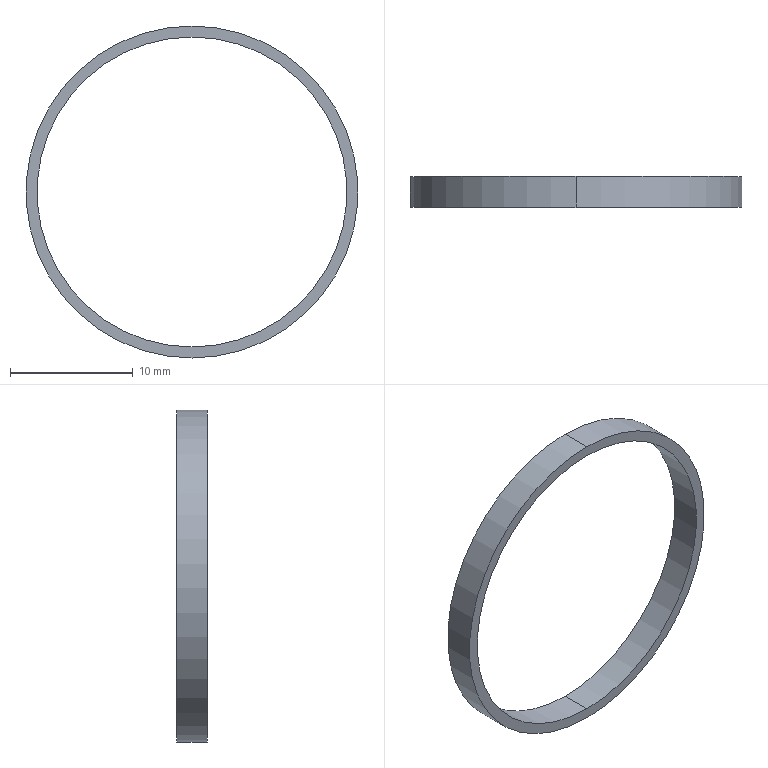Part | SolidWorks | features Extrusion 1 | 1 solid | 6 faces | box 27 x 2.5 x 27 mm | volume 184.49 mm3 | cylinder 4 | plane 2 | commonest cylinder face diameters 25.2 x2 27 x2
STEP:
#1=CARTESIAN_POINT('',(0.,2.5,-12.6));
#2=VERTEX_POINT('',#1);
#3=CARTESIAN_POINT('',(0.,2.5,12.6));
#4=VERTEX_POINT('',#3);
#5=CARTESIAN_POINT('',(0.,2.5,0.));
#6=DIRECTION('',(0.,1.,0.));
#7=DIRECTION('',(0.,0.,1.));
#8=AXIS2_PLACEMENT_3D('',#5,#6,#7);
#9=CIRCLE('',#8,12.6);
#10=EDGE_CURVE('',#2,#4,#9,.T.);
#11=ORIENTED_EDGE('',*,*,#10,.T.);
#12=CARTESIAN_POINT('',(0.,0.,12.6));
#13=VERTEX_POINT('',#12);
#14=CARTESIAN_POINT('',(0.,2.5,12.6));
#15=DIRECTION('',(0.,-1.,0.));
#16=VECTOR('',#15,1000.);
#17=LINE('',#14,#16);
#18=EDGE_CURVE('',#4,#13,#17,.T.);
#19=ORIENTED_EDGE('',*,*,#18,.T.);
#20=CARTESIAN_POINT('',(0.,0.,-12.6));
#21=VERTEX_POINT('',#20);
#22=CARTESIAN_POINT('',(0.,0.,0.));
#23=DIRECTION('',(0.,1.,0.));
#24=DIRECTION('',(0.,0.,1.));
#25=AXIS2_PLACEMENT_3D('',#22,#23,#24);
#26=CIRCLE('',#25,12.6);
#27=EDGE_CURVE('',#21,#13,#26,.T.);
#28=ORIENTED_EDGE('',*,*,#27,.F.);
#29=CARTESIAN_POINT('',(0.,2.5,-12.6));
#30=DIRECTION('',(0.,-1.,0.));
#31=VECTOR('',#30,1000.);
#32=LINE('',#29,#31);
#33=EDGE_CURVE('',#2,#21,#32,.T.);
#34=ORIENTED_EDGE('',*,*,#33,.F.);
#35=EDGE_LOOP('',(#11,#19,#28,#34));
#36=FACE_OUTER_BOUND('',#35,.T.);
#37=CARTESIAN_POINT('',(0.,2.5,0.));
#38=DIRECTION('',(0.,-1.,0.));
#39=DIRECTION('',(0.,0.,-1.));
#40=AXIS2_PLACEMENT_3D('',#37,#38,#39);
#41=CYLINDRICAL_SURFACE('',#40,12.6);
#42=ADVANCED_FACE('',(#36),#41,.F.);
#43=CARTESIAN_POINT('',(0.,2.5,13.5));
#44=VERTEX_POINT('',#43);
#45=CARTESIAN_POINT('',(0.,2.5,-13.5));
#46=VERTEX_POINT('',#45);
#47=CARTESIAN_POINT('',(0.,2.5,0.));
#48=DIRECTION('',(0.,1.,0.));
#49=DIRECTION('',(0.,0.,1.));
#50=AXIS2_PLACEMENT_3D('',#47,#48,#49);
#51=CIRCLE('',#50,13.5);
#52=EDGE_CURVE('',#44,#46,#51,.T.);
#53=ORIENTED_EDGE('',*,*,#52,.F.);
#54=CARTESIAN_POINT('',(0.,0.,13.5));
#55=VERTEX_POINT('',#54);
#56=CARTESIAN_POINT('',(0.,2.5,13.5));
#57=DIRECTION('',(0.,-1.,0.));
#58=VECTOR('',#57,1000.);
#59=LINE('',#56,#58);
#60=EDGE_CURVE('',#44,#55,#59,.T.);
#61=ORIENTED_EDGE('',*,*,#60,.T.);
#62=CARTESIAN_POINT('',(0.,0.,-13.5));
#63=VERTEX_POINT('',#62);
#64=CARTESIAN_POINT('',(0.,0.,0.));
#65=DIRECTION('',(0.,1.,0.));
#66=DIRECTION('',(0.,0.,1.));
#67=AXIS2_PLACEMENT_3D('',#64,#65,#66);
#68=CIRCLE('',#67,13.5);
#69=EDGE_CURVE('',#55,#63,#68,.T.);
#70=ORIENTED_EDGE('',*,*,#69,.T.);
#71=CARTESIAN_POINT('',(0.,2.5,-13.5));
#72=DIRECTION('',(0.,-1.,0.));
#73=VECTOR('',#72,1000.);
#74=LINE('',#71,#73);
#75=EDGE_CURVE('',#46,#63,#74,.T.);
#76=ORIENTED_EDGE('',*,*,#75,.F.);
#77=EDGE_LOOP('',(#53,#61,#70,#76));
#78=FACE_OUTER_BOUND('',#77,.T.);
#79=CARTESIAN_POINT('',(0.,2.5,0.));
#80=DIRECTION('',(0.,-1.,0.));
#81=DIRECTION('',(0.,0.,-1.));
#82=AXIS2_PLACEMENT_3D('',#79,#80,#81);
#83=CYLINDRICAL_SURFACE('',#82,13.5);
#84=ADVANCED_FACE('',(#78),#83,.T.);
#85=CARTESIAN_POINT('',(0.,2.5,0.));
#86=DIRECTION('',(0.,1.,0.));
#87=DIRECTION('',(0.,0.,1.));
#88=AXIS2_PLACEMENT_3D('',#85,#86,#87);
#89=CIRCLE('',#88,13.5);
#90=EDGE_CURVE('',#46,#44,#89,.T.);
#91=ORIENTED_EDGE('',*,*,#90,.T.);
#92=ORIENTED_EDGE('',*,*,#52,.T.);
#93=EDGE_LOOP('',(#91,#92));
#94=FACE_OUTER_BOUND('',#93,.T.);
#95=ORIENTED_EDGE('',*,*,#10,.F.);
#96=CARTESIAN_POINT('',(0.,2.5,0.));
#97=DIRECTION('',(0.,1.,0.));
#98=DIRECTION('',(0.,0.,1.));
#99=AXIS2_PLACEMENT_3D('',#96,#97,#98);
#100=CIRCLE('',#99,12.6);
#101=EDGE_CURVE('',#4,#2,#100,.T.);
#102=ORIENTED_EDGE('',*,*,#101,.F.);
#103=EDGE_LOOP('',(#95,#102));
#104=FACE_BOUND('',#103,.T.);
#105=CARTESIAN_POINT('',(0.,2.5,0.));
#106=DIRECTION('',(0.,1.,0.));
#107=DIRECTION('',(0.,0.,1.));
#108=AXIS2_PLACEMENT_3D('',#105,#106,#107);
#109=PLANE('',#108);
#110=ADVANCED_FACE('',(#94,#104),#109,.T.);
#111=CARTESIAN_POINT('',(0.,0.,0.));
#112=DIRECTION('',(0.,1.,0.));
#113=DIRECTION('',(0.,0.,1.));
#114=AXIS2_PLACEMENT_3D('',#111,#112,#113);
#115=CIRCLE('',#114,13.5);
#116=EDGE_CURVE('',#63,#55,#115,.T.);
#117=ORIENTED_EDGE('',*,*,#116,.F.);
#118=ORIENTED_EDGE('',*,*,#69,.F.);
#119=EDGE_LOOP('',(#117,#118));
#120=FACE_OUTER_BOUND('',#119,.T.);
#121=ORIENTED_EDGE('',*,*,#27,.T.);
#122=CARTESIAN_POINT('',(0.,0.,0.));
#123=DIRECTION('',(0.,1.,0.));
#124=DIRECTION('',(0.,0.,1.));
#125=AXIS2_PLACEMENT_3D('',#122,#123,#124);
#126=CIRCLE('',#125,12.6);
#127=EDGE_CURVE('',#13,#21,#126,.T.);
#128=ORIENTED_EDGE('',*,*,#127,.T.);
#129=EDGE_LOOP('',(#121,#128));
#130=FACE_BOUND('',#129,.T.);
#131=CARTESIAN_POINT('',(0.,0.,0.));
#132=DIRECTION('',(0.,1.,0.));
#133=DIRECTION('',(0.,0.,1.));
#134=AXIS2_PLACEMENT_3D('',#131,#132,#133);
#135=PLANE('',#134);
#136=ADVANCED_FACE('',(#120,#130),#135,.F.);
#137=ORIENTED_EDGE('',*,*,#60,.F.);
#138=ORIENTED_EDGE('',*,*,#90,.F.);
#139=ORIENTED_EDGE('',*,*,#75,.T.);
#140=ORIENTED_EDGE('',*,*,#116,.T.);
#141=EDGE_LOOP('',(#137,#138,#139,#140));
#142=FACE_OUTER_BOUND('',#141,.T.);
#143=CARTESIAN_POINT('',(0.,2.5,0.));
#144=DIRECTION('',(0.,-1.,0.));
#145=DIRECTION('',(0.,0.,-1.));
#146=AXIS2_PLACEMENT_3D('',#143,#144,#145);
#147=CYLINDRICAL_SURFACE('',#146,13.5);
#148=ADVANCED_FACE('',(#142),#147,.T.);
#149=ORIENTED_EDGE('',*,*,#18,.F.);
#150=ORIENTED_EDGE('',*,*,#101,.T.);
#151=ORIENTED_EDGE('',*,*,#33,.T.);
#152=ORIENTED_EDGE('',*,*,#127,.F.);
#153=EDGE_LOOP('',(#149,#150,#151,#152));
#154=FACE_OUTER_BOUND('',#153,.T.);
#155=CARTESIAN_POINT('',(0.,2.5,0.));
#156=DIRECTION('',(0.,-1.,0.));
#157=DIRECTION('',(0.,0.,-1.));
#158=AXIS2_PLACEMENT_3D('',#155,#156,#157);
#159=CYLINDRICAL_SURFACE('',#158,12.6);
#160=ADVANCED_FACE('',(#154),#159,.F.);
#161=CLOSED_SHELL('',(#42,#84,#110,#136,#148,#160));
#162=MANIFOLD_SOLID_BREP('',#161);
#163=CARTESIAN_POINT('',(0.,0.,0.));
#164=DIRECTION('',(0.,0.,1.));
#165=DIRECTION('',(1.,0.,0.));
#166=AXIS2_PLACEMENT_3D('',#163,#164,#165);
#167=(LENGTH_UNIT()NAMED_UNIT(*)SI_UNIT(.MILLI.,.METRE.));
#168=UNCERTAINTY_MEASURE_WITH_UNIT(LENGTH_MEASURE(0.00001),#167,'','');
#169=(NAMED_UNIT(*)PLANE_ANGLE_UNIT()SI_UNIT($,.RADIAN.));
#170=(NAMED_UNIT(*)SI_UNIT($,.STERADIAN.)SOLID_ANGLE_UNIT());
#171=(GEOMETRIC_REPRESENTATION_CONTEXT(3)GLOBAL_UNCERTAINTY_ASSIGNED_CONTEXT((#168))GLOBAL_UNIT_ASSIGNED_CONTEXT((#167,#169,#170))REPRESENTATION_CONTEXT('',''));
#172=ADVANCED_BREP_SHAPE_REPRESENTATION('',(#162,#166),#171);